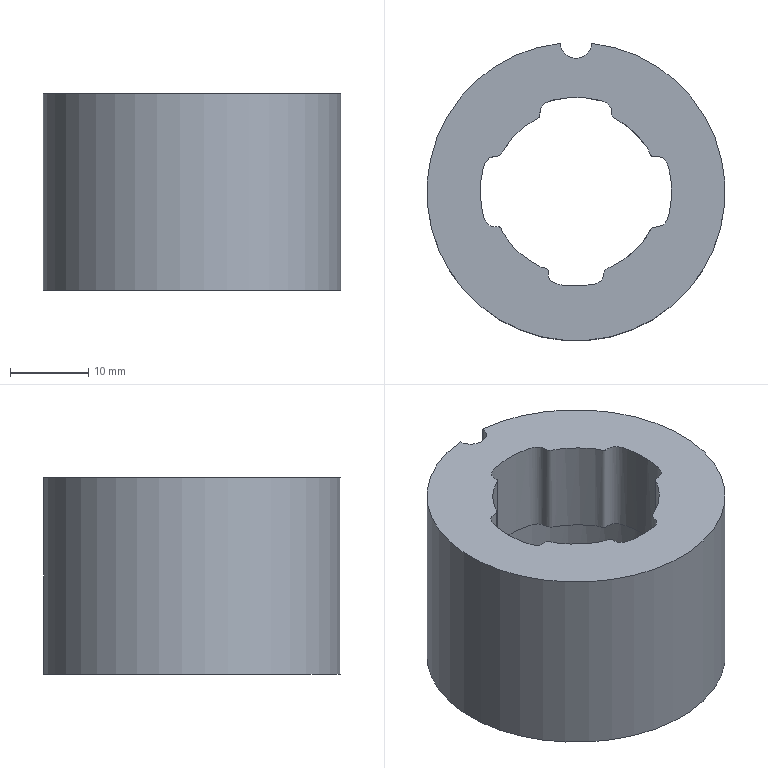Part | NX | features solid 2 | 1 solid | 9 faces | box 38 x 37.895 x 25 mm | volume 15842 mm3 | plane 3 | cylinder 3 | spline 3 | commonest cylinder face diameters 4 x1 26.6 x1 38 x1
STEP:
#1=CARTESIAN_POINT('',(-1.997,-534.501,-62.));
#2=VERTEX_POINT('',#1);
#3=CARTESIAN_POINT('',(1.997,-534.501,-62.));
#4=VERTEX_POINT('',#3);
#5=CARTESIAN_POINT('',(0.,-534.396,-62.));
#6=DIRECTION('',(0.,0.,1.));
#7=DIRECTION('',(0.,1.,0.));
#8=AXIS2_PLACEMENT_3D('',#5,#6,#7);
#9=CIRCLE('',#8,2.);
#10=EDGE_CURVE('',#2,#4,#9,.T.);
#11=ORIENTED_EDGE('',*,*,#10,.F.);
#12=CARTESIAN_POINT('',(0.,-553.396,-62.));
#13=DIRECTION('',(0.,0.,1.));
#14=DIRECTION('',(0.,1.,0.));
#15=AXIS2_PLACEMENT_3D('',#12,#13,#14);
#16=CIRCLE('',#15,19.);
#17=EDGE_CURVE('',#2,#4,#16,.T.);
#18=ORIENTED_EDGE('',*,*,#17,.T.);
#19=EDGE_LOOP('',(#11,#18));
#20=FACE_BOUND('',#19,.T.);
#21=CARTESIAN_POINT('',(-4.646,-543.907,-62.));
#22=VERTEX_POINT('',#21);
#23=CARTESIAN_POINT('',(4.638,-562.891,-62.));
#24=VERTEX_POINT('',#23);
#25=CARTESIAN_POINT('',(-4.646,-543.907,-62.));
#26=CARTESIAN_POINT('',(-5.364,-544.249,-62.));
#27=CARTESIAN_POINT('',(-6.366,-544.873,-62.));
#28=CARTESIAN_POINT('',(-7.566,-545.924,-62.));
#29=CARTESIAN_POINT('',(-8.351,-546.799,-62.));
#30=CARTESIAN_POINT('',(-8.955,-547.58,-62.));
#31=CARTESIAN_POINT('',(-9.328,-548.268,-62.));
#32=CARTESIAN_POINT('',(-9.746,-549.011,-62.));
#33=CARTESIAN_POINT('',(-10.949,-548.781,-62.));
#34=CARTESIAN_POINT('',(-11.748,-549.875,-62.));
#35=CARTESIAN_POINT('',(-11.97,-551.056,-62.));
#36=CARTESIAN_POINT('',(-12.173,-552.259,-62.));
#37=CARTESIAN_POINT('',(-12.222,-553.463,-62.));
#38=CARTESIAN_POINT('',(-12.161,-554.661,-62.));
#39=CARTESIAN_POINT('',(-11.947,-555.854,-62.));
#40=CARTESIAN_POINT('',(-11.713,-557.049,-62.));
#41=CARTESIAN_POINT('',(-10.985,-557.902,-62.));
#42=CARTESIAN_POINT('',(-10.248,-557.912,-62.));
#43=CARTESIAN_POINT('',(-9.833,-557.849,-62.));
#44=CARTESIAN_POINT('',(-9.551,-558.008,-62.));
#45=CARTESIAN_POINT('',(-9.448,-558.308,-62.));
#46=CARTESIAN_POINT('',(-9.299,-558.683,-62.));
#47=CARTESIAN_POINT('',(-9.017,-559.096,-62.));
#48=CARTESIAN_POINT('',(-8.662,-559.579,-62.));
#49=CARTESIAN_POINT('',(-8.191,-560.223,-62.));
#50=CARTESIAN_POINT('',(-7.507,-560.933,-62.));
#51=CARTESIAN_POINT('',(-6.61,-561.702,-62.));
#52=CARTESIAN_POINT('',(-5.802,-562.284,-62.));
#53=CARTESIAN_POINT('',(-5.096,-562.642,-62.));
#54=CARTESIAN_POINT('',(-4.601,-562.981,-62.));
#55=CARTESIAN_POINT('',(-4.13,-563.105,-62.));
#56=CARTESIAN_POINT('',(-3.73,-563.172,-62.));
#57=CARTESIAN_POINT('',(-3.522,-563.404,-62.));
#58=CARTESIAN_POINT('',(-3.564,-563.715,-62.));
#59=CARTESIAN_POINT('',(-3.574,-564.105,-62.));
#60=CARTESIAN_POINT('',(-3.381,-564.582,-62.));
#61=CARTESIAN_POINT('',(-2.911,-564.963,-62.));
#62=CARTESIAN_POINT('',(-2.189,-565.289,-62.));
#63=CARTESIAN_POINT('',(-0.812,-565.382,-62.));
#64=CARTESIAN_POINT('',(0.7425,-565.433,-62.));
#65=CARTESIAN_POINT('',(2.111,-565.272,-62.));
#66=CARTESIAN_POINT('',(2.853,-565.013,-62.));
#67=CARTESIAN_POINT('',(3.326,-564.634,-62.));
#68=CARTESIAN_POINT('',(3.531,-564.081,-62.));
#69=CARTESIAN_POINT('',(3.582,-563.228,-62.));
#70=CARTESIAN_POINT('',(4.274,-563.049,-62.));
#71=CARTESIAN_POINT('',(4.638,-562.891,-62.));
#72=B_SPLINE_CURVE_WITH_KNOTS('',3,(#25,#26,#27,#28,#29,#30,#31,#32,#33,#34,#35,#36,#37,#38,#39,#40,#41,#42,#43,#44,#45,#46,#47,#48,#49,#50,#51,#52,#53,#54,#55,#56,#57,#58,#59,#60,#61,#62,#63,#64,#65,#66,#67,#68,#69,#70,#71),.UNSPECIFIED.,.F.,.F.,(4,1,1,1,1,1,1,1,1,1,1,1,1,1,1,1,1,1,1,1,1,1,1,1,1,1,1,1,1,1,1,1,1,1,1,1,1,1,1,1,1,1,1,1,4),(0.,0.002363,0.003545,0.004727,0.005909,0.006499,0.00709,0.008272,0.009454,0.01064,0.01182,0.013,0.01418,0.01536,0.01654,0.01773,0.01832,0.01861,0.01891,0.0192,0.0195,0.02009,0.02068,0.02127,0.02245,0.02363,0.02482,0.02541,0.026,0.02659,0.02688,0.02718,0.02747,0.02777,0.02836,0.02895,0.02954,0.03072,0.03309,0.03427,0.03486,0.03545,0.03604,0.03663,0.03781),.UNSPECIFIED.);
#73=EDGE_CURVE('',#22,#24,#72,.T.);
#74=ORIENTED_EDGE('',*,*,#73,.F.);
#75=CARTESIAN_POINT('',(-4.613,-543.695,-62.));
#76=VERTEX_POINT('',#75);
#77=CARTESIAN_POINT('',(-4.646,-543.907,-62.));
#78=CARTESIAN_POINT('',(-4.578,-543.875,-62.));
#79=CARTESIAN_POINT('',(-4.612,-543.768,-62.));
#80=CARTESIAN_POINT('',(-4.613,-543.695,-62.));
#81=B_SPLINE_CURVE_WITH_KNOTS('',3,(#77,#78,#79,#80),.UNSPECIFIED.,.F.,.F.,(4,4),(0.,0.0002225),.UNSPECIFIED.);
#82=EDGE_CURVE('',#22,#76,#81,.T.);
#83=ORIENTED_EDGE('',*,*,#82,.T.);
#84=CARTESIAN_POINT('',(4.638,-562.891,-62.));
#85=CARTESIAN_POINT('',(5.384,-562.566,-62.));
#86=CARTESIAN_POINT('',(6.74,-561.682,-62.));
#87=CARTESIAN_POINT('',(8.138,-560.244,-62.));
#88=CARTESIAN_POINT('',(9.041,-559.149,-62.));
#89=CARTESIAN_POINT('',(9.347,-558.393,-62.));
#90=CARTESIAN_POINT('',(9.769,-557.918,-62.));
#91=CARTESIAN_POINT('',(10.402,-557.914,-62.));
#92=CARTESIAN_POINT('',(11.187,-557.709,-62.));
#93=CARTESIAN_POINT('',(11.771,-556.831,-62.));
#94=CARTESIAN_POINT('',(11.983,-555.664,-62.));
#95=CARTESIAN_POINT('',(12.169,-554.492,-62.));
#96=CARTESIAN_POINT('',(12.211,-553.307,-62.));
#97=CARTESIAN_POINT('',(12.153,-552.134,-62.));
#98=CARTESIAN_POINT('',(11.941,-550.984,-62.));
#99=CARTESIAN_POINT('',(11.778,-549.989,-62.));
#100=CARTESIAN_POINT('',(11.326,-549.334,-62.));
#101=CARTESIAN_POINT('',(10.841,-548.961,-62.));
#102=CARTESIAN_POINT('',(10.271,-548.843,-62.));
#103=CARTESIAN_POINT('',(9.582,-548.995,-62.));
#104=CARTESIAN_POINT('',(9.369,-548.335,-62.));
#105=CARTESIAN_POINT('',(9.13,-547.821,-62.));
#106=CARTESIAN_POINT('',(8.732,-547.361,-62.));
#107=CARTESIAN_POINT('',(8.287,-546.695,-62.));
#108=CARTESIAN_POINT('',(7.602,-545.976,-62.));
#109=CARTESIAN_POINT('',(6.715,-545.191,-62.));
#110=CARTESIAN_POINT('',(5.912,-544.569,-62.));
#111=CARTESIAN_POINT('',(5.199,-544.226,-62.));
#112=CARTESIAN_POINT('',(4.465,-543.789,-62.));
#113=CARTESIAN_POINT('',(4.645,-542.591,-62.));
#114=CARTESIAN_POINT('',(3.587,-541.837,-62.));
#115=CARTESIAN_POINT('',(2.424,-541.622,-62.));
#116=CARTESIAN_POINT('',(1.26,-541.428,-62.));
#117=CARTESIAN_POINT('',(0.08941,-541.369,-62.));
#118=CARTESIAN_POINT('',(-1.088,-541.407,-62.));
#119=CARTESIAN_POINT('',(-2.268,-541.578,-62.));
#120=CARTESIAN_POINT('',(-3.429,-541.8,-62.));
#121=CARTESIAN_POINT('',(-4.524,-542.442,-62.));
#122=CARTESIAN_POINT('',(-4.615,-543.298,-62.));
#123=CARTESIAN_POINT('',(-4.613,-543.695,-62.));
#124=B_SPLINE_CURVE_WITH_KNOTS('',3,(#84,#85,#86,#87,#88,#89,#90,#91,#92,#93,#94,#95,#96,#97,#98,#99,#100,#101,#102,#103,#104,#105,#106,#107,#108,#109,#110,#111,#112,#113,#114,#115,#116,#117,#118,#119,#120,#121,#122,#123),.UNSPECIFIED.,.F.,.F.,(4,1,1,1,1,1,1,1,1,1,1,1,1,1,1,1,1,1,1,1,1,1,1,1,1,1,1,1,1,1,1,1,1,1,1,1,1,4),(0.,0.002408,0.004815,0.006019,0.006621,0.007223,0.007825,0.008427,0.009631,0.01083,0.01204,0.01324,0.01445,0.01565,0.01685,0.01746,0.01806,0.01866,0.01926,0.01986,0.02047,0.02107,0.02167,0.02287,0.02408,0.02528,0.02588,0.02648,0.02769,0.02889,0.0301,0.0313,0.0325,0.03371,0.03491,0.03612,0.03732,0.03852),.UNSPECIFIED.);
#125=EDGE_CURVE('',#24,#76,#124,.T.);
#126=ORIENTED_EDGE('',*,*,#125,.F.);
#127=EDGE_LOOP('',(#74,#83,#126));
#128=FACE_BOUND('',#127,.T.);
#129=CARTESIAN_POINT('',(0.,-543.896,-62.));
#130=DIRECTION('',(0.,0.,1.));
#131=DIRECTION('',(0.,1.,0.));
#132=AXIS2_PLACEMENT_3D('',#129,#130,#131);
#133=PLANE('',#132);
#134=ADVANCED_FACE('',(#20,#128),#133,.T.);
#135=CARTESIAN_POINT('',(13.3,-553.396,-74.));
#136=VERTEX_POINT('',#135);
#137=CARTESIAN_POINT('',(0.,-553.396,-74.));
#138=DIRECTION('',(0.,0.,1.));
#139=DIRECTION('',(1.,0.,0.));
#140=AXIS2_PLACEMENT_3D('',#137,#138,#139);
#141=CIRCLE('',#140,13.3);
#142=EDGE_CURVE('',#136,#136,#141,.T.);
#143=ORIENTED_EDGE('',*,*,#142,.F.);
#144=EDGE_LOOP('',(#143));
#145=FACE_BOUND('',#144,.T.);
#146=CARTESIAN_POINT('',(-4.646,-543.907,-74.));
#147=VERTEX_POINT('',#146);
#148=CARTESIAN_POINT('',(-4.613,-543.695,-74.));
#149=VERTEX_POINT('',#148);
#150=CARTESIAN_POINT('',(-4.613,-543.695,-74.));
#151=CARTESIAN_POINT('',(-4.612,-543.768,-74.));
#152=CARTESIAN_POINT('',(-4.579,-543.875,-74.));
#153=CARTESIAN_POINT('',(-4.646,-543.907,-74.));
#154=B_SPLINE_CURVE_WITH_KNOTS('',3,(#150,#151,#152,#153),.UNSPECIFIED.,.F.,.F.,(4,4),(0.0004607,0.0006819),.UNSPECIFIED.);
#155=EDGE_CURVE('',#147,#149,#154,.F.);
#156=ORIENTED_EDGE('',*,*,#155,.F.);
#157=CARTESIAN_POINT('',(4.638,-562.891,-74.));
#158=VERTEX_POINT('',#157);
#159=CARTESIAN_POINT('',(-4.646,-543.907,-74.));
#160=CARTESIAN_POINT('',(-5.364,-544.249,-74.));
#161=CARTESIAN_POINT('',(-6.366,-544.873,-74.));
#162=CARTESIAN_POINT('',(-7.566,-545.924,-74.));
#163=CARTESIAN_POINT('',(-8.351,-546.799,-74.));
#164=CARTESIAN_POINT('',(-8.955,-547.58,-74.));
#165=CARTESIAN_POINT('',(-9.328,-548.268,-74.));
#166=CARTESIAN_POINT('',(-9.746,-549.011,-74.));
#167=CARTESIAN_POINT('',(-10.949,-548.781,-74.));
#168=CARTESIAN_POINT('',(-11.748,-549.875,-74.));
#169=CARTESIAN_POINT('',(-11.97,-551.056,-74.));
#170=CARTESIAN_POINT('',(-12.173,-552.259,-74.));
#171=CARTESIAN_POINT('',(-12.222,-553.463,-74.));
#172=CARTESIAN_POINT('',(-12.161,-554.661,-74.));
#173=CARTESIAN_POINT('',(-11.947,-555.854,-74.));
#174=CARTESIAN_POINT('',(-11.713,-557.049,-74.));
#175=CARTESIAN_POINT('',(-10.985,-557.902,-74.));
#176=CARTESIAN_POINT('',(-10.248,-557.912,-74.));
#177=CARTESIAN_POINT('',(-9.833,-557.849,-74.));
#178=CARTESIAN_POINT('',(-9.551,-558.008,-74.));
#179=CARTESIAN_POINT('',(-9.448,-558.308,-74.));
#180=CARTESIAN_POINT('',(-9.299,-558.683,-74.));
#181=CARTESIAN_POINT('',(-9.017,-559.096,-74.));
#182=CARTESIAN_POINT('',(-8.662,-559.579,-74.));
#183=CARTESIAN_POINT('',(-8.191,-560.223,-74.));
#184=CARTESIAN_POINT('',(-7.507,-560.933,-74.));
#185=CARTESIAN_POINT('',(-6.61,-561.702,-74.));
#186=CARTESIAN_POINT('',(-5.802,-562.284,-74.));
#187=CARTESIAN_POINT('',(-5.096,-562.642,-74.));
#188=CARTESIAN_POINT('',(-4.601,-562.981,-74.));
#189=CARTESIAN_POINT('',(-4.13,-563.105,-74.));
#190=CARTESIAN_POINT('',(-3.73,-563.172,-74.));
#191=CARTESIAN_POINT('',(-3.522,-563.404,-74.));
#192=CARTESIAN_POINT('',(-3.564,-563.715,-74.));
#193=CARTESIAN_POINT('',(-3.574,-564.105,-74.));
#194=CARTESIAN_POINT('',(-3.381,-564.582,-74.));
#195=CARTESIAN_POINT('',(-2.911,-564.963,-74.));
#196=CARTESIAN_POINT('',(-2.189,-565.289,-74.));
#197=CARTESIAN_POINT('',(-0.812,-565.382,-74.));
#198=CARTESIAN_POINT('',(0.7425,-565.433,-74.));
#199=CARTESIAN_POINT('',(2.111,-565.272,-74.));
#200=CARTESIAN_POINT('',(2.853,-565.013,-74.));
#201=CARTESIAN_POINT('',(3.326,-564.634,-74.));
#202=CARTESIAN_POINT('',(3.531,-564.081,-74.));
#203=CARTESIAN_POINT('',(3.582,-563.228,-74.));
#204=CARTESIAN_POINT('',(4.274,-563.049,-74.));
#205=CARTESIAN_POINT('',(4.638,-562.891,-74.));
#206=B_SPLINE_CURVE_WITH_KNOTS('',3,(#159,#160,#161,#162,#163,#164,#165,#166,#167,#168,#169,#170,#171,#172,#173,#174,#175,#176,#177,#178,#179,#180,#181,#182,#183,#184,#185,#186,#187,#188,#189,#190,#191,#192,#193,#194,#195,#196,#197,#198,#199,#200,#201,#202,#203,#204,#205),.UNSPECIFIED.,.F.,.F.,(4,1,1,1,1,1,1,1,1,1,1,1,1,1,1,1,1,1,1,1,1,1,1,1,1,1,1,1,1,1,1,1,1,1,1,1,1,1,1,1,1,1,1,1,4),(0.,0.002363,0.003545,0.004727,0.005909,0.006499,0.00709,0.008272,0.009454,0.01064,0.01182,0.013,0.01418,0.01536,0.01654,0.01773,0.01832,0.01861,0.01891,0.0192,0.0195,0.02009,0.02068,0.02127,0.02245,0.02363,0.02482,0.02541,0.026,0.02659,0.02688,0.02718,0.02747,0.02777,0.02836,0.02895,0.02954,0.03072,0.03309,0.03427,0.03486,0.03545,0.03604,0.03663,0.03781),.UNSPECIFIED.);
#207=EDGE_CURVE('',#147,#158,#206,.T.);
#208=ORIENTED_EDGE('',*,*,#207,.T.);
#209=CARTESIAN_POINT('',(4.638,-562.891,-74.));
#210=CARTESIAN_POINT('',(5.349,-562.581,-74.));
#211=CARTESIAN_POINT('',(6.339,-561.929,-74.));
#212=CARTESIAN_POINT('',(7.496,-560.927,-74.));
#213=CARTESIAN_POINT('',(8.161,-560.229,-74.));
#214=CARTESIAN_POINT('',(8.63,-559.606,-74.));
#215=CARTESIAN_POINT('',(8.996,-559.146,-74.));
#216=CARTESIAN_POINT('',(9.274,-558.639,-74.));
#217=CARTESIAN_POINT('',(9.52,-558.059,-74.));
#218=CARTESIAN_POINT('',(10.12,-557.91,-74.));
#219=CARTESIAN_POINT('',(10.906,-557.851,-74.));
#220=CARTESIAN_POINT('',(11.691,-557.15,-74.));
#221=CARTESIAN_POINT('',(11.914,-555.969,-74.));
#222=CARTESIAN_POINT('',(12.133,-554.835,-74.));
#223=CARTESIAN_POINT('',(12.209,-553.662,-74.));
#224=CARTESIAN_POINT('',(12.18,-552.494,-74.));
#225=CARTESIAN_POINT('',(12.029,-551.338,-74.));
#226=CARTESIAN_POINT('',(11.843,-550.377,-74.));
#227=CARTESIAN_POINT('',(11.571,-549.631,-74.));
#228=CARTESIAN_POINT('',(11.159,-549.182,-74.));
#229=CARTESIAN_POINT('',(10.628,-548.872,-74.));
#230=CARTESIAN_POINT('',(10.126,-548.886,-74.));
#231=CARTESIAN_POINT('',(9.704,-548.924,-74.));
#232=CARTESIAN_POINT('',(9.407,-548.624,-74.));
#233=CARTESIAN_POINT('',(9.318,-548.115,-74.));
#234=CARTESIAN_POINT('',(8.959,-547.636,-74.));
#235=CARTESIAN_POINT('',(8.48,-546.988,-74.));
#236=CARTESIAN_POINT('',(7.845,-546.217,-74.));
#237=CARTESIAN_POINT('',(7.13,-545.526,-74.));
#238=CARTESIAN_POINT('',(6.495,-545.038,-74.));
#239=CARTESIAN_POINT('',(6.015,-544.675,-74.));
#240=CARTESIAN_POINT('',(5.504,-544.347,-74.));
#241=CARTESIAN_POINT('',(4.923,-544.125,-74.));
#242=CARTESIAN_POINT('',(4.549,-543.62,-74.));
#243=CARTESIAN_POINT('',(4.559,-542.987,-74.));
#244=CARTESIAN_POINT('',(4.324,-542.402,-74.));
#245=CARTESIAN_POINT('',(3.656,-541.879,-74.));
#246=CARTESIAN_POINT('',(2.648,-541.665,-74.));
#247=CARTESIAN_POINT('',(1.45,-541.448,-74.));
#248=CARTESIAN_POINT('',(0.245,-541.371,-74.));
#249=CARTESIAN_POINT('',(-0.9604,-541.397,-74.));
#250=CARTESIAN_POINT('',(-2.173,-541.558,-74.));
#251=CARTESIAN_POINT('',(-3.366,-541.784,-74.));
#252=CARTESIAN_POINT('',(-4.513,-542.404,-74.));
#253=CARTESIAN_POINT('',(-4.615,-543.288,-74.));
#254=CARTESIAN_POINT('',(-4.613,-543.695,-74.));
#255=B_SPLINE_CURVE_WITH_KNOTS('',3,(#209,#210,#211,#212,#213,#214,#215,#216,#217,#218,#219,#220,#221,#222,#223,#224,#225,#226,#227,#228,#229,#230,#231,#232,#233,#234,#235,#236,#237,#238,#239,#240,#241,#242,#243,#244,#245,#246,#247,#248,#249,#250,#251,#252,#253,#254),.UNSPECIFIED.,.F.,.F.,(4,1,1,1,1,1,1,1,1,1,1,1,1,1,1,1,1,1,1,1,1,1,1,1,1,1,1,1,1,1,1,1,1,1,1,1,1,1,1,1,1,1,1,4),(0.06249,0.06482,0.06598,0.06714,0.06773,0.06831,0.06889,0.06947,0.07005,0.07063,0.0718,0.07296,0.07412,0.07528,0.07645,0.07761,0.07877,0.07935,0.07993,0.08052,0.0811,0.08139,0.08168,0.08226,0.08284,0.08342,0.08459,0.08575,0.08633,0.08691,0.08749,0.08807,0.08866,0.08924,0.08982,0.0904,0.09156,0.09272,0.09389,0.09505,0.09621,0.09738,0.09854,0.0997),.UNSPECIFIED.);
#256=EDGE_CURVE('',#158,#149,#255,.T.);
#257=ORIENTED_EDGE('',*,*,#256,.T.);
#258=EDGE_LOOP('',(#156,#208,#257));
#259=FACE_BOUND('',#258,.T.);
#260=CARTESIAN_POINT('',(0.,-553.396,-74.));
#261=DIRECTION('',(0.,0.,1.));
#262=DIRECTION('',(0.,1.,0.));
#263=AXIS2_PLACEMENT_3D('',#260,#261,#262);
#264=PLANE('',#263);
#265=ADVANCED_FACE('',(#145,#259),#264,.F.);
#266=ORIENTED_EDGE('',*,*,#10,.T.);
#267=CARTESIAN_POINT('',(1.997,-534.501,-87.));
#268=VERTEX_POINT('',#267);
#269=CARTESIAN_POINT('',(1.997,-534.501,-87.));
#270=DIRECTION('',(0.,0.,1.));
#271=VECTOR('',#270,1000.);
#272=LINE('',#269,#271);
#273=EDGE_CURVE('',#268,#4,#272,.T.);
#274=ORIENTED_EDGE('',*,*,#273,.F.);
#275=CARTESIAN_POINT('',(-1.997,-534.501,-87.));
#276=VERTEX_POINT('',#275);
#277=CARTESIAN_POINT('',(0.,-534.396,-87.));
#278=DIRECTION('',(0.,0.,1.));
#279=DIRECTION('',(0.,1.,0.));
#280=AXIS2_PLACEMENT_3D('',#277,#278,#279);
#281=CIRCLE('',#280,2.);
#282=EDGE_CURVE('',#276,#268,#281,.T.);
#283=ORIENTED_EDGE('',*,*,#282,.F.);
#284=CARTESIAN_POINT('',(-1.997,-534.501,-87.));
#285=DIRECTION('',(0.,0.,1.));
#286=VECTOR('',#285,1000.);
#287=LINE('',#284,#286);
#288=EDGE_CURVE('',#2,#276,#287,.F.);
#289=ORIENTED_EDGE('',*,*,#288,.F.);
#290=EDGE_LOOP('',(#266,#274,#283,#289));
#291=FACE_BOUND('',#290,.T.);
#292=CARTESIAN_POINT('',(0.,-534.396,-87.));
#293=DIRECTION('',(0.,0.,1.));
#294=DIRECTION('',(0.,1.,0.));
#295=AXIS2_PLACEMENT_3D('',#292,#293,#294);
#296=CYLINDRICAL_SURFACE('',#295,2.);
#297=ADVANCED_FACE('',(#291),#296,.F.);
#298=ORIENTED_EDGE('',*,*,#17,.F.);
#299=ORIENTED_EDGE('',*,*,#288,.T.);
#300=CARTESIAN_POINT('',(0.,-553.396,-87.));
#301=DIRECTION('',(0.,0.,1.));
#302=DIRECTION('',(0.,1.,0.));
#303=AXIS2_PLACEMENT_3D('',#300,#301,#302);
#304=CIRCLE('',#303,19.);
#305=EDGE_CURVE('',#276,#268,#304,.T.);
#306=ORIENTED_EDGE('',*,*,#305,.T.);
#307=ORIENTED_EDGE('',*,*,#273,.T.);
#308=EDGE_LOOP('',(#298,#299,#306,#307));
#309=FACE_BOUND('',#308,.T.);
#310=CARTESIAN_POINT('',(0.,-553.396,-87.));
#311=DIRECTION('',(0.,0.,1.));
#312=DIRECTION('',(0.,1.,0.));
#313=AXIS2_PLACEMENT_3D('',#310,#311,#312);
#314=CYLINDRICAL_SURFACE('',#313,19.);
#315=ADVANCED_FACE('',(#309),#314,.T.);
#316=CARTESIAN_POINT('',(0.,-540.096,-87.));
#317=VERTEX_POINT('',#316);
#318=CARTESIAN_POINT('',(0.,-553.396,-87.));
#319=DIRECTION('',(0.,0.,1.));
#320=DIRECTION('',(0.,1.,0.));
#321=AXIS2_PLACEMENT_3D('',#318,#319,#320);
#322=CIRCLE('',#321,13.3);
#323=EDGE_CURVE('',#317,#317,#322,.T.);
#324=ORIENTED_EDGE('',*,*,#323,.T.);
#325=EDGE_LOOP('',(#324));
#326=FACE_BOUND('',#325,.T.);
#327=ORIENTED_EDGE('',*,*,#282,.T.);
#328=ORIENTED_EDGE('',*,*,#305,.F.);
#329=EDGE_LOOP('',(#327,#328));
#330=FACE_BOUND('',#329,.T.);
#331=CARTESIAN_POINT('',(0.,-543.896,-87.));
#332=DIRECTION('',(0.,0.,1.));
#333=DIRECTION('',(0.,1.,0.));
#334=AXIS2_PLACEMENT_3D('',#331,#332,#333);
#335=PLANE('',#334);
#336=ADVANCED_FACE('',(#326,#330),#335,.F.);
#337=ORIENTED_EDGE('',*,*,#323,.F.);
#338=EDGE_LOOP('',(#337));
#339=FACE_BOUND('',#338,.T.);
#340=ORIENTED_EDGE('',*,*,#142,.T.);
#341=EDGE_LOOP('',(#340));
#342=FACE_BOUND('',#341,.T.);
#343=CARTESIAN_POINT('',(0.,-553.396,-87.));
#344=DIRECTION('',(0.,0.,1.));
#345=DIRECTION('',(0.,1.,0.));
#346=AXIS2_PLACEMENT_3D('',#343,#344,#345);
#347=CYLINDRICAL_SURFACE('',#346,13.3);
#348=ADVANCED_FACE('',(#339,#342),#347,.F.);
#349=CARTESIAN_POINT('',(-4.646,-543.907,-1164.976));
#350=DIRECTION('',(0.,0.,1.));
#351=VECTOR('',#350,1000.);
#352=LINE('',#349,#351);
#353=EDGE_CURVE('',#147,#22,#352,.T.);
#354=ORIENTED_EDGE('',*,*,#353,.F.);
#355=ORIENTED_EDGE('',*,*,#155,.T.);
#356=CARTESIAN_POINT('',(-4.613,-543.695,-1164.976));
#357=DIRECTION('',(0.,0.,1.));
#358=VECTOR('',#357,1000.);
#359=LINE('',#356,#358);
#360=EDGE_CURVE('',#149,#76,#359,.T.);
#361=ORIENTED_EDGE('',*,*,#360,.T.);
#362=ORIENTED_EDGE('',*,*,#82,.F.);
#363=EDGE_LOOP('',(#354,#355,#361,#362));
#364=FACE_BOUND('',#363,.T.);
#365=CARTESIAN_POINT('',(-4.646,-543.907,-74.));
#366=CARTESIAN_POINT('',(-4.646,-543.907,-62.));
#367=CARTESIAN_POINT('',(-4.597,-543.884,-74.));
#368=CARTESIAN_POINT('',(-4.597,-543.884,-62.));
#369=CARTESIAN_POINT('',(-4.634,-543.892,-74.));
#370=CARTESIAN_POINT('',(-4.634,-543.892,-62.));
#371=CARTESIAN_POINT('',(-4.612,-543.759,-74.));
#372=CARTESIAN_POINT('',(-4.612,-543.759,-62.));
#373=CARTESIAN_POINT('',(-4.613,-543.695,-74.));
#374=CARTESIAN_POINT('',(-4.613,-543.695,-62.));
#375=B_SPLINE_SURFACE_WITH_KNOTS('',3,1,((#365,#366),(#367,#368),(#369,#370),(#371,#372),(#373,#374)),.SURF_OF_LINEAR_EXTRUSION.,.F.,.F.,.F.,(4,1,4),(2,2),(-0.00000479,0.5,1.),(0.,1.),.UNSPECIFIED.);
#376=ADVANCED_FACE('',(#364),#375,.T.);
#377=ORIENTED_EDGE('',*,*,#125,.T.);
#378=ORIENTED_EDGE('',*,*,#360,.F.);
#379=ORIENTED_EDGE('',*,*,#256,.F.);
#380=CARTESIAN_POINT('',(4.638,-562.891,-1164.976));
#381=DIRECTION('',(0.,0.,1.));
#382=VECTOR('',#381,1000.);
#383=LINE('',#380,#382);
#384=EDGE_CURVE('',#158,#24,#383,.T.);
#385=ORIENTED_EDGE('',*,*,#384,.T.);
#386=EDGE_LOOP('',(#377,#378,#379,#385));
#387=FACE_BOUND('',#386,.T.);
#388=CARTESIAN_POINT('',(4.638,-562.891,-74.));
#389=CARTESIAN_POINT('',(4.638,-562.891,-62.));
#390=CARTESIAN_POINT('',(5.398,-562.56,-74.));
#391=CARTESIAN_POINT('',(5.398,-562.56,-62.));
#392=CARTESIAN_POINT('',(6.376,-561.898,-74.));
#393=CARTESIAN_POINT('',(6.376,-561.898,-62.));
#394=CARTESIAN_POINT('',(7.586,-560.854,-74.));
#395=CARTESIAN_POINT('',(7.586,-560.854,-62.));
#396=CARTESIAN_POINT('',(8.379,-559.941,-74.));
#397=CARTESIAN_POINT('',(8.379,-559.941,-62.));
#398=CARTESIAN_POINT('',(8.993,-559.21,-74.));
#399=CARTESIAN_POINT('',(8.993,-559.21,-62.));
#400=CARTESIAN_POINT('',(9.361,-558.41,-74.));
#401=CARTESIAN_POINT('',(9.361,-558.41,-62.));
#402=CARTESIAN_POINT('',(9.63,-558.016,-74.));
#403=CARTESIAN_POINT('',(9.63,-558.016,-62.));
#404=CARTESIAN_POINT('',(10.093,-557.922,-74.));
#405=CARTESIAN_POINT('',(10.093,-557.922,-62.));
#406=CARTESIAN_POINT('',(10.734,-557.858,-74.));
#407=CARTESIAN_POINT('',(10.734,-557.858,-62.));
#408=CARTESIAN_POINT('',(11.315,-557.538,-74.));
#409=CARTESIAN_POINT('',(11.315,-557.538,-62.));
#410=CARTESIAN_POINT('',(11.756,-556.807,-74.));
#411=CARTESIAN_POINT('',(11.756,-556.807,-62.));
#412=CARTESIAN_POINT('',(11.949,-555.835,-74.));
#413=CARTESIAN_POINT('',(11.949,-555.835,-62.));
#414=CARTESIAN_POINT('',(12.151,-554.667,-74.));
#415=CARTESIAN_POINT('',(12.151,-554.667,-62.));
#416=CARTESIAN_POINT('',(12.211,-553.482,-74.));
#417=CARTESIAN_POINT('',(12.211,-553.482,-62.));
#418=CARTESIAN_POINT('',(12.168,-552.295,-74.));
#419=CARTESIAN_POINT('',(12.168,-552.295,-62.));
#420=CARTESIAN_POINT('',(11.974,-551.127,-74.));
#421=CARTESIAN_POINT('',(11.974,-551.127,-62.));
#422=CARTESIAN_POINT('',(11.819,-550.138,-74.));
#423=CARTESIAN_POINT('',(11.819,-550.138,-62.));
#424=CARTESIAN_POINT('',(11.404,-549.415,-74.));
#425=CARTESIAN_POINT('',(11.404,-549.415,-62.));
#426=CARTESIAN_POINT('',(10.927,-548.993,-74.));
#427=CARTESIAN_POINT('',(10.927,-548.993,-62.));
#428=CARTESIAN_POINT('',(10.259,-548.843,-74.));
#429=CARTESIAN_POINT('',(10.259,-548.843,-62.));
#430=CARTESIAN_POINT('',(9.63,-548.959,-74.));
#431=CARTESIAN_POINT('',(9.63,-548.959,-62.));
#432=CARTESIAN_POINT('',(9.434,-548.579,-74.));
#433=CARTESIAN_POINT('',(9.434,-548.579,-62.));
#434=CARTESIAN_POINT('',(9.189,-547.881,-74.));
#435=CARTESIAN_POINT('',(9.189,-547.881,-62.));
#436=CARTESIAN_POINT('',(8.811,-547.47,-74.));
#437=CARTESIAN_POINT('',(8.811,-547.47,-62.));
#438=CARTESIAN_POINT('',(8.368,-546.805,-74.));
#439=CARTESIAN_POINT('',(8.368,-546.805,-62.));
#440=CARTESIAN_POINT('',(7.694,-546.067,-74.));
#441=CARTESIAN_POINT('',(7.694,-546.067,-62.));
#442=CARTESIAN_POINT('',(6.8,-545.256,-74.));
#443=CARTESIAN_POINT('',(6.8,-545.256,-62.));
#444=CARTESIAN_POINT('',(6.035,-544.656,-74.));
#445=CARTESIAN_POINT('',(6.035,-544.656,-62.));
#446=CARTESIAN_POINT('',(5.285,-544.258,-74.));
#447=CARTESIAN_POINT('',(5.285,-544.258,-62.));
#448=CARTESIAN_POINT('',(4.778,-543.995,-74.));
#449=CARTESIAN_POINT('',(4.778,-543.995,-62.));
#450=CARTESIAN_POINT('',(4.585,-543.637,-74.));
#451=CARTESIAN_POINT('',(4.585,-543.637,-62.));
#452=CARTESIAN_POINT('',(4.557,-543.038,-74.));
#453=CARTESIAN_POINT('',(4.557,-543.038,-62.));
#454=CARTESIAN_POINT('',(4.338,-542.408,-74.));
#455=CARTESIAN_POINT('',(4.338,-542.408,-62.));
#456=CARTESIAN_POINT('',(3.822,-542.005,-74.));
#457=CARTESIAN_POINT('',(3.822,-542.005,-62.));
#458=CARTESIAN_POINT('',(3.239,-541.806,-74.));
#459=CARTESIAN_POINT('',(3.239,-541.806,-62.));
#460=CARTESIAN_POINT('',(2.458,-541.623,-74.));
#461=CARTESIAN_POINT('',(2.458,-541.623,-62.));
#462=CARTESIAN_POINT('',(1.47,-541.453,-74.));
#463=CARTESIAN_POINT('',(1.47,-541.453,-62.));
#464=CARTESIAN_POINT('',(0.2675,-541.371,-74.));
#465=CARTESIAN_POINT('',(0.2675,-541.371,-62.));
#466=CARTESIAN_POINT('',(-0.9363,-541.395,-74.));
#467=CARTESIAN_POINT('',(-0.9363,-541.395,-62.));
#468=CARTESIAN_POINT('',(-2.139,-541.552,-74.));
#469=CARTESIAN_POINT('',(-2.139,-541.552,-62.));
#470=CARTESIAN_POINT('',(-3.291,-541.765,-74.));
#471=CARTESIAN_POINT('',(-3.291,-541.765,-62.));
#472=CARTESIAN_POINT('',(-4.517,-542.38,-74.));
#473=CARTESIAN_POINT('',(-4.517,-542.38,-62.));
#474=CARTESIAN_POINT('',(-4.615,-543.292,-74.));
#475=CARTESIAN_POINT('',(-4.615,-543.292,-62.));
#476=CARTESIAN_POINT('',(-4.613,-543.695,-74.));
#477=CARTESIAN_POINT('',(-4.613,-543.695,-62.));
#478=B_SPLINE_SURFACE_WITH_KNOTS('',3,1,((#388,#389),(#390,#391),(#392,#393),(#394,#395),(#396,#397),(#398,#399),(#400,#401),(#402,#403),(#404,#405),(#406,#407),(#408,#409),(#410,#411),(#412,#413),(#414,#415),(#416,#417),(#418,#419),(#420,#421),(#422,#423),(#424,#425),(#426,#427),(#428,#429),(#430,#431),(#432,#433),(#434,#435),(#436,#437),(#438,#439),(#440,#441),(#442,#443),(#444,#445),(#446,#447),(#448,#449),(#450,#451),(#452,#453),(#454,#455),(#456,#457),(#458,#459),(#460,#461),(#462,#463),(#464,#465),(#466,#467),(#468,#469),(#470,#471),(#472,#473),(#474,#475),(#476,#477)),.SURF_OF_LINEAR_EXTRUSION.,.F.,.F.,.F.,(4,1,1,1,1,1,1,1,1,1,1,1,1,1,1,1,1,1,1,1,1,1,1,1,1,1,1,1,1,1,1,1,1,1,1,1,1,1,1,1,1,1,4),(2,2),(0.,0.0625,0.09375,0.125,0.1563,0.1719,0.1875,0.2031,0.2188,0.2344,0.25,0.2812,0.3125,0.3437,0.375,0.4062,0.4375,0.4531,0.4687,0.4844,0.5,0.5156,0.5312,0.5469,0.5625,0.5937,0.625,0.6562,0.6719,0.6875,0.7031,0.7187,0.7344,0.75,0.7656,0.7812,0.8125,0.8437,0.875,0.9062,0.9375,0.9687,1.),(0.,1.),.UNSPECIFIED.);
#479=ADVANCED_FACE('',(#387),#478,.F.);
#480=ORIENTED_EDGE('',*,*,#73,.T.);
#481=ORIENTED_EDGE('',*,*,#384,.F.);
#482=ORIENTED_EDGE('',*,*,#207,.F.);
#483=ORIENTED_EDGE('',*,*,#353,.T.);
#484=EDGE_LOOP('',(#480,#481,#482,#483));
#485=FACE_BOUND('',#484,.T.);
#486=CARTESIAN_POINT('',(-4.646,-543.907,-74.));
#487=CARTESIAN_POINT('',(-4.646,-543.907,-62.));
#488=CARTESIAN_POINT('',(-5.372,-544.252,-74.));
#489=CARTESIAN_POINT('',(-5.372,-544.252,-62.));
#490=CARTESIAN_POINT('',(-6.399,-544.896,-74.));
#491=CARTESIAN_POINT('',(-6.399,-544.896,-62.));
#492=CARTESIAN_POINT('',(-7.601,-545.957,-74.));
#493=CARTESIAN_POINT('',(-7.601,-545.957,-62.));
#494=CARTESIAN_POINT('',(-8.401,-546.861,-74.));
#495=CARTESIAN_POINT('',(-8.401,-546.861,-62.));
#496=CARTESIAN_POINT('',(-9.,-547.641,-74.));
#497=CARTESIAN_POINT('',(-9.,-547.641,-62.));
#498=CARTESIAN_POINT('',(-9.383,-548.386,-74.));
#499=CARTESIAN_POINT('',(-9.383,-548.386,-62.));
#500=CARTESIAN_POINT('',(-9.669,-548.804,-74.));
#501=CARTESIAN_POINT('',(-9.669,-548.804,-62.));
#502=CARTESIAN_POINT('',(-10.1,-548.916,-74.));
#503=CARTESIAN_POINT('',(-10.1,-548.916,-62.));
#504=CARTESIAN_POINT('',(-10.787,-548.921,-74.));
#505=CARTESIAN_POINT('',(-10.787,-548.921,-62.));
#506=CARTESIAN_POINT('',(-11.343,-549.299,-74.));
#507=CARTESIAN_POINT('',(-11.343,-549.299,-62.));
#508=CARTESIAN_POINT('',(-11.763,-550.035,-74.));
#509=CARTESIAN_POINT('',(-11.763,-550.035,-62.));
#510=CARTESIAN_POINT('',(-11.966,-551.016,-74.));
#511=CARTESIAN_POINT('',(-11.966,-551.016,-62.));
#512=CARTESIAN_POINT('',(-12.163,-552.186,-74.));
#513=CARTESIAN_POINT('',(-12.163,-552.186,-62.));
#514=CARTESIAN_POINT('',(-12.222,-553.376,-74.));
#515=CARTESIAN_POINT('',(-12.222,-553.376,-62.));
#516=CARTESIAN_POINT('',(-12.17,-554.569,-74.));
#517=CARTESIAN_POINT('',(-12.17,-554.569,-62.));
#518=CARTESIAN_POINT('',(-11.968,-555.733,-74.));
#519=CARTESIAN_POINT('',(-11.968,-555.733,-62.));
#520=CARTESIAN_POINT('',(-11.795,-556.735,-74.));
#521=CARTESIAN_POINT('',(-11.795,-556.735,-62.));
#522=CARTESIAN_POINT('',(-11.359,-557.439,-74.));
#523=CARTESIAN_POINT('',(-11.359,-557.439,-62.));
#524=CARTESIAN_POINT('',(-10.881,-557.89,-74.));
#525=CARTESIAN_POINT('',(-10.881,-557.89,-62.));
#526=CARTESIAN_POINT('',(-10.13,-557.907,-74.));
#527=CARTESIAN_POINT('',(-10.13,-557.907,-62.));
#528=CARTESIAN_POINT('',(-9.616,-557.839,-74.));
#529=CARTESIAN_POINT('',(-9.616,-557.839,-62.));
#530=CARTESIAN_POINT('',(-9.436,-558.372,-74.));
#531=CARTESIAN_POINT('',(-9.436,-558.372,-62.));
#532=CARTESIAN_POINT('',(-9.132,-558.972,-74.));
#533=CARTESIAN_POINT('',(-9.132,-558.972,-62.));
#534=CARTESIAN_POINT('',(-8.777,-559.399,-74.));
#535=CARTESIAN_POINT('',(-8.777,-559.399,-62.));
#536=CARTESIAN_POINT('',(-8.32,-560.079,-74.));
#537=CARTESIAN_POINT('',(-8.32,-560.079,-62.));
#538=CARTESIAN_POINT('',(-7.638,-560.8,-74.));
#539=CARTESIAN_POINT('',(-7.638,-560.8,-62.));
#540=CARTESIAN_POINT('',(-6.733,-561.604,-74.));
#541=CARTESIAN_POINT('',(-6.733,-561.604,-62.));
#542=CARTESIAN_POINT('',(-5.944,-562.206,-74.));
#543=CARTESIAN_POINT('',(-5.944,-562.206,-62.));
#544=CARTESIAN_POINT('',(-5.2,-562.579,-74.));
#545=CARTESIAN_POINT('',(-5.2,-562.579,-62.));
#546=CARTESIAN_POINT('',(-4.76,-562.899,-74.));
#547=CARTESIAN_POINT('',(-4.76,-562.899,-62.));
#548=CARTESIAN_POINT('',(-4.084,-563.123,-74.));
#549=CARTESIAN_POINT('',(-4.084,-563.123,-62.));
#550=CARTESIAN_POINT('',(-3.506,-563.224,-74.));
#551=CARTESIAN_POINT('',(-3.506,-563.224,-62.));
#552=CARTESIAN_POINT('',(-3.591,-563.735,-74.));
#553=CARTESIAN_POINT('',(-3.591,-563.735,-62.));
#554=CARTESIAN_POINT('',(-3.498,-564.471,-74.));
#555=CARTESIAN_POINT('',(-3.498,-564.471,-62.));
#556=CARTESIAN_POINT('',(-2.999,-564.9,-74.));
#557=CARTESIAN_POINT('',(-2.999,-564.9,-62.));
#558=CARTESIAN_POINT('',(-2.264,-565.287,-74.));
#559=CARTESIAN_POINT('',(-2.264,-565.287,-62.));
#560=CARTESIAN_POINT('',(-1.225,-565.345,-74.));
#561=CARTESIAN_POINT('',(-1.225,-565.345,-62.));
#562=CARTESIAN_POINT('',(-0.0303,-565.434,-74.));
#563=CARTESIAN_POINT('',(-0.0303,-565.434,-62.));
#564=CARTESIAN_POINT('',(1.179,-565.377,-74.));
#565=CARTESIAN_POINT('',(1.179,-565.377,-62.));
#566=CARTESIAN_POINT('',(2.184,-565.264,-74.));
#567=CARTESIAN_POINT('',(2.184,-565.264,-62.));
#568=CARTESIAN_POINT('',(2.969,-564.957,-74.));
#569=CARTESIAN_POINT('',(2.969,-564.957,-62.));
#570=CARTESIAN_POINT('',(3.439,-564.479,-74.));
#571=CARTESIAN_POINT('',(3.439,-564.479,-62.));
#572=CARTESIAN_POINT('',(3.545,-563.804,-74.));
#573=CARTESIAN_POINT('',(3.545,-563.804,-62.));
#574=CARTESIAN_POINT('',(3.683,-563.216,-74.));
#575=CARTESIAN_POINT('',(3.683,-563.216,-62.));
#576=CARTESIAN_POINT('',(4.256,-563.057,-74.));
#577=CARTESIAN_POINT('',(4.256,-563.057,-62.));
#578=CARTESIAN_POINT('',(4.638,-562.891,-74.));
#579=CARTESIAN_POINT('',(4.638,-562.891,-62.));
#580=B_SPLINE_SURFACE_WITH_KNOTS('',3,1,((#486,#487),(#488,#489),(#490,#491),(#492,#493),(#494,#495),(#496,#497),(#498,#499),(#500,#501),(#502,#503),(#504,#505),(#506,#507),(#508,#509),(#510,#511),(#512,#513),(#514,#515),(#516,#517),(#518,#519),(#520,#521),(#522,#523),(#524,#525),(#526,#527),(#528,#529),(#530,#531),(#532,#533),(#534,#535),(#536,#537),(#538,#539),(#540,#541),(#542,#543),(#544,#545),(#546,#547),(#548,#549),(#550,#551),(#552,#553),(#554,#555),(#556,#557),(#558,#559),(#560,#561),(#562,#563),(#564,#565),(#566,#567),(#568,#569),(#570,#571),(#572,#573),(#574,#575),(#576,#577),(#578,#579)),.SURF_OF_LINEAR_EXTRUSION.,.F.,.F.,.F.,(4,1,1,1,1,1,1,1,1,1,1,1,1,1,1,1,1,1,1,1,1,1,1,1,1,1,1,1,1,1,1,1,1,1,1,1,1,1,1,1,1,1,1,1,4),(2,2),(0.,0.0625,0.09375,0.125,0.1562,0.1719,0.1875,0.2031,0.2187,0.2344,0.25,0.2812,0.3125,0.3438,0.375,0.4063,0.4375,0.4531,0.4688,0.4844,0.5,0.5156,0.5313,0.5469,0.5625,0.5938,0.625,0.6563,0.6719,0.6875,0.7031,0.7188,0.7344,0.75,0.7656,0.7813,0.8125,0.8438,0.875,0.9063,0.9219,0.9375,0.9531,0.9688,1.),(0.,1.),.UNSPECIFIED.);
#581=ADVANCED_FACE('',(#485),#580,.F.);
#582=CLOSED_SHELL('',(#134,#265,#297,#315,#336,#348,#376,#479,#581));
#583=MANIFOLD_SOLID_BREP('',#582);
#584=(LENGTH_UNIT()NAMED_UNIT(*)SI_UNIT(.MILLI.,.METRE.));
#585=UNCERTAINTY_MEASURE_WITH_UNIT(LENGTH_MEASURE(0.0508),#584,'','');
#586=(NAMED_UNIT(*)PLANE_ANGLE_UNIT()SI_UNIT($,.RADIAN.));
#587=(NAMED_UNIT(*)SI_UNIT($,.STERADIAN.)SOLID_ANGLE_UNIT());
#588=(GEOMETRIC_REPRESENTATION_CONTEXT(3)GLOBAL_UNCERTAINTY_ASSIGNED_CONTEXT((#585))GLOBAL_UNIT_ASSIGNED_CONTEXT((#584,#586,#587))REPRESENTATION_CONTEXT('',''));
#589=ADVANCED_BREP_SHAPE_REPRESENTATION('',(#583),#588);